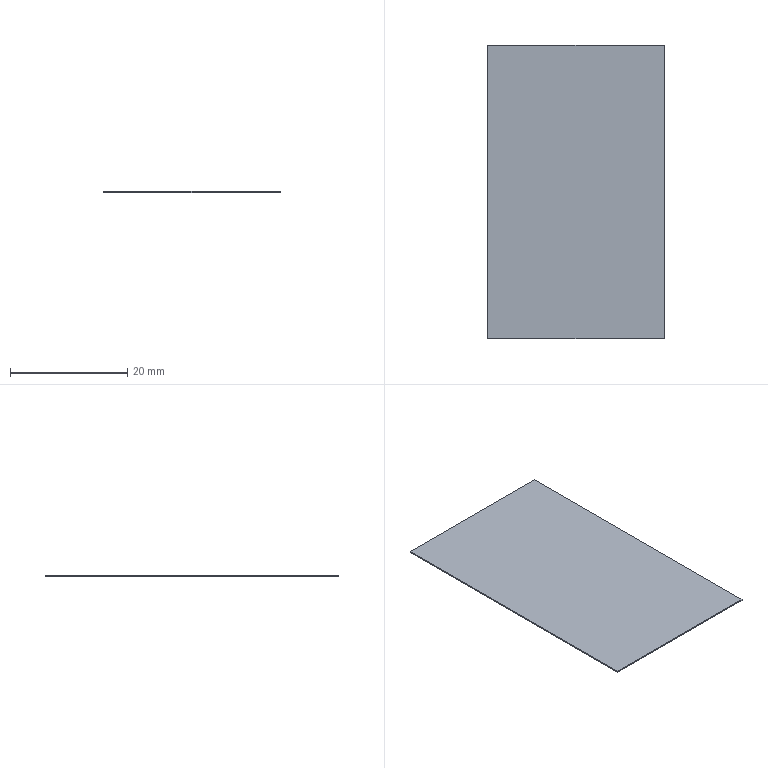Part | SolidWorks | features Extrusion 1 | 1 solid | 6 faces | box 30 x 50 x 0.2 mm | volume 300 mm3 | plane 6
STEP:
#1=CARTESIAN_POINT('',(-15.,-25.,0.));
#2=VERTEX_POINT('',#1);
#3=CARTESIAN_POINT('',(15.,-25.,0.));
#4=VERTEX_POINT('',#3);
#5=CARTESIAN_POINT('',(0.,-25.,0.));
#6=DIRECTION('',(1.,0.,0.));
#7=VECTOR('',#6,1000.);
#8=LINE('',#5,#7);
#9=EDGE_CURVE('',#2,#4,#8,.T.);
#10=ORIENTED_EDGE('',*,*,#9,.T.);
#11=CARTESIAN_POINT('',(15.,-25.,0.2));
#12=VERTEX_POINT('',#11);
#13=CARTESIAN_POINT('',(15.,-25.,0.2));
#14=DIRECTION('',(0.,0.,-1.));
#15=VECTOR('',#14,1000.);
#16=LINE('',#13,#15);
#17=EDGE_CURVE('',#12,#4,#16,.T.);
#18=ORIENTED_EDGE('',*,*,#17,.F.);
#19=CARTESIAN_POINT('',(-15.,-25.,0.2));
#20=VERTEX_POINT('',#19);
#21=CARTESIAN_POINT('',(0.,-25.,0.2));
#22=DIRECTION('',(1.,0.,0.));
#23=VECTOR('',#22,1000.);
#24=LINE('',#21,#23);
#25=EDGE_CURVE('',#20,#12,#24,.T.);
#26=ORIENTED_EDGE('',*,*,#25,.F.);
#27=CARTESIAN_POINT('',(-15.,-25.,0.2));
#28=DIRECTION('',(0.,0.,-1.));
#29=VECTOR('',#28,1000.);
#30=LINE('',#27,#29);
#31=EDGE_CURVE('',#20,#2,#30,.T.);
#32=ORIENTED_EDGE('',*,*,#31,.T.);
#33=EDGE_LOOP('',(#10,#18,#26,#32));
#34=FACE_OUTER_BOUND('',#33,.T.);
#35=CARTESIAN_POINT('',(0.,-25.,0.2));
#36=DIRECTION('',(0.,1.,0.));
#37=DIRECTION('',(-1.,0.,0.));
#38=AXIS2_PLACEMENT_3D('',#35,#36,#37);
#39=PLANE('',#38);
#40=ADVANCED_FACE('',(#34),#39,.F.);
#41=CARTESIAN_POINT('',(15.,25.,0.));
#42=VERTEX_POINT('',#41);
#43=CARTESIAN_POINT('',(15.,0.,0.));
#44=DIRECTION('',(0.,1.,0.));
#45=VECTOR('',#44,1000.);
#46=LINE('',#43,#45);
#47=EDGE_CURVE('',#4,#42,#46,.T.);
#48=ORIENTED_EDGE('',*,*,#47,.T.);
#49=CARTESIAN_POINT('',(15.,25.,0.2));
#50=VERTEX_POINT('',#49);
#51=CARTESIAN_POINT('',(15.,25.,0.2));
#52=DIRECTION('',(0.,0.,-1.));
#53=VECTOR('',#52,1000.);
#54=LINE('',#51,#53);
#55=EDGE_CURVE('',#50,#42,#54,.T.);
#56=ORIENTED_EDGE('',*,*,#55,.F.);
#57=CARTESIAN_POINT('',(15.,0.,0.2));
#58=DIRECTION('',(0.,1.,0.));
#59=VECTOR('',#58,1000.);
#60=LINE('',#57,#59);
#61=EDGE_CURVE('',#12,#50,#60,.T.);
#62=ORIENTED_EDGE('',*,*,#61,.F.);
#63=ORIENTED_EDGE('',*,*,#17,.T.);
#64=EDGE_LOOP('',(#48,#56,#62,#63));
#65=FACE_OUTER_BOUND('',#64,.T.);
#66=CARTESIAN_POINT('',(15.,0.,0.2));
#67=DIRECTION('',(-1.,0.,0.));
#68=DIRECTION('',(0.,0.,1.));
#69=AXIS2_PLACEMENT_3D('',#66,#67,#68);
#70=PLANE('',#69);
#71=ADVANCED_FACE('',(#65),#70,.F.);
#72=CARTESIAN_POINT('',(-15.,25.,0.));
#73=VERTEX_POINT('',#72);
#74=CARTESIAN_POINT('',(0.,25.,0.));
#75=DIRECTION('',(1.,0.,0.));
#76=VECTOR('',#75,1000.);
#77=LINE('',#74,#76);
#78=EDGE_CURVE('',#73,#42,#77,.T.);
#79=ORIENTED_EDGE('',*,*,#78,.F.);
#80=CARTESIAN_POINT('',(-15.,25.,0.2));
#81=VERTEX_POINT('',#80);
#82=CARTESIAN_POINT('',(-15.,25.,0.2));
#83=DIRECTION('',(0.,0.,-1.));
#84=VECTOR('',#83,1000.);
#85=LINE('',#82,#84);
#86=EDGE_CURVE('',#81,#73,#85,.T.);
#87=ORIENTED_EDGE('',*,*,#86,.F.);
#88=CARTESIAN_POINT('',(0.,25.,0.2));
#89=DIRECTION('',(1.,0.,0.));
#90=VECTOR('',#89,1000.);
#91=LINE('',#88,#90);
#92=EDGE_CURVE('',#81,#50,#91,.T.);
#93=ORIENTED_EDGE('',*,*,#92,.T.);
#94=ORIENTED_EDGE('',*,*,#55,.T.);
#95=EDGE_LOOP('',(#79,#87,#93,#94));
#96=FACE_OUTER_BOUND('',#95,.T.);
#97=CARTESIAN_POINT('',(0.,25.,0.2));
#98=DIRECTION('',(0.,1.,0.));
#99=DIRECTION('',(0.,0.,1.));
#100=AXIS2_PLACEMENT_3D('',#97,#98,#99);
#101=PLANE('',#100);
#102=ADVANCED_FACE('',(#96),#101,.T.);
#103=CARTESIAN_POINT('',(-15.,0.,0.));
#104=DIRECTION('',(0.,1.,0.));
#105=VECTOR('',#104,1000.);
#106=LINE('',#103,#105);
#107=EDGE_CURVE('',#2,#73,#106,.T.);
#108=ORIENTED_EDGE('',*,*,#107,.F.);
#109=ORIENTED_EDGE('',*,*,#31,.F.);
#110=CARTESIAN_POINT('',(-15.,0.,0.2));
#111=DIRECTION('',(0.,1.,0.));
#112=VECTOR('',#111,1000.);
#113=LINE('',#110,#112);
#114=EDGE_CURVE('',#20,#81,#113,.T.);
#115=ORIENTED_EDGE('',*,*,#114,.T.);
#116=ORIENTED_EDGE('',*,*,#86,.T.);
#117=EDGE_LOOP('',(#108,#109,#115,#116));
#118=FACE_OUTER_BOUND('',#117,.T.);
#119=CARTESIAN_POINT('',(-15.,0.,0.2));
#120=DIRECTION('',(-1.,0.,0.));
#121=DIRECTION('',(0.,0.,1.));
#122=AXIS2_PLACEMENT_3D('',#119,#120,#121);
#123=PLANE('',#122);
#124=ADVANCED_FACE('',(#118),#123,.T.);
#125=ORIENTED_EDGE('',*,*,#25,.T.);
#126=ORIENTED_EDGE('',*,*,#61,.T.);
#127=ORIENTED_EDGE('',*,*,#92,.F.);
#128=ORIENTED_EDGE('',*,*,#114,.F.);
#129=EDGE_LOOP('',(#125,#126,#127,#128));
#130=FACE_OUTER_BOUND('',#129,.T.);
#131=CARTESIAN_POINT('',(0.,0.,0.2));
#132=DIRECTION('',(0.,0.,1.));
#133=DIRECTION('',(1.,0.,0.));
#134=AXIS2_PLACEMENT_3D('',#131,#132,#133);
#135=PLANE('',#134);
#136=ADVANCED_FACE('',(#130),#135,.T.);
#137=ORIENTED_EDGE('',*,*,#9,.F.);
#138=ORIENTED_EDGE('',*,*,#107,.T.);
#139=ORIENTED_EDGE('',*,*,#78,.T.);
#140=ORIENTED_EDGE('',*,*,#47,.F.);
#141=EDGE_LOOP('',(#137,#138,#139,#140));
#142=FACE_OUTER_BOUND('',#141,.T.);
#143=CARTESIAN_POINT('',(0.,0.,0.));
#144=DIRECTION('',(0.,0.,1.));
#145=DIRECTION('',(1.,0.,0.));
#146=AXIS2_PLACEMENT_3D('',#143,#144,#145);
#147=PLANE('',#146);
#148=ADVANCED_FACE('',(#142),#147,.F.);
#149=CLOSED_SHELL('',(#40,#71,#102,#124,#136,#148));
#150=MANIFOLD_SOLID_BREP('',#149);
#151=CARTESIAN_POINT('',(0.,0.,0.));
#152=DIRECTION('',(0.,0.,1.));
#153=DIRECTION('',(1.,0.,0.));
#154=AXIS2_PLACEMENT_3D('',#151,#152,#153);
#155=(LENGTH_UNIT()NAMED_UNIT(*)SI_UNIT(.MILLI.,.METRE.));
#156=UNCERTAINTY_MEASURE_WITH_UNIT(LENGTH_MEASURE(0.00001),#155,'','');
#157=(NAMED_UNIT(*)PLANE_ANGLE_UNIT()SI_UNIT($,.RADIAN.));
#158=(NAMED_UNIT(*)SI_UNIT($,.STERADIAN.)SOLID_ANGLE_UNIT());
#159=(GEOMETRIC_REPRESENTATION_CONTEXT(3)GLOBAL_UNCERTAINTY_ASSIGNED_CONTEXT((#156))GLOBAL_UNIT_ASSIGNED_CONTEXT((#155,#157,#158))REPRESENTATION_CONTEXT('',''));
#160=ADVANCED_BREP_SHAPE_REPRESENTATION('',(#150,#154),#159);